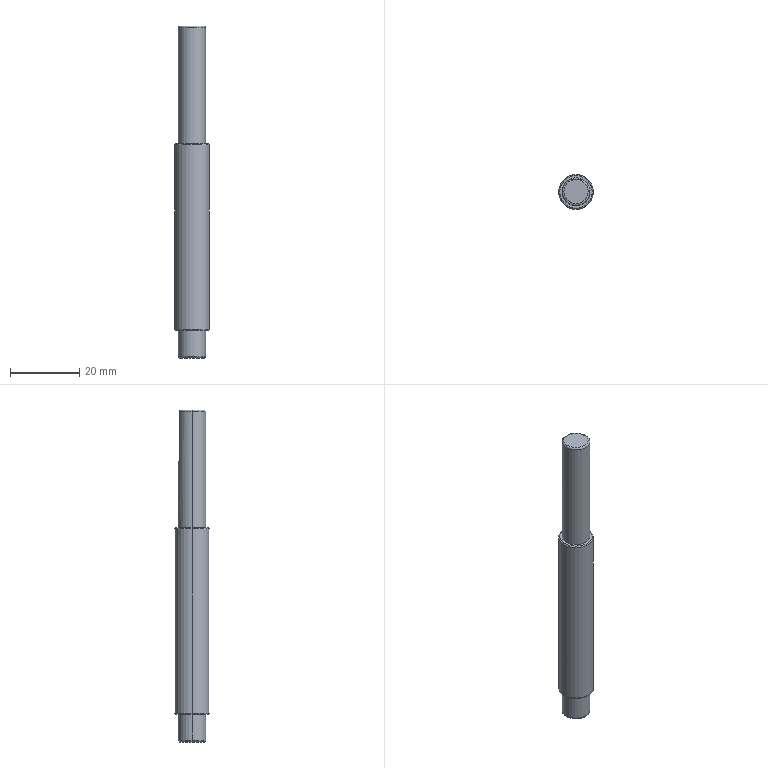Part | NX | features BREP 1 | 1 solid | 21 faces | box 10 x 10 x 95.8 mm | volume 6313 mm3 | torus 9 | cylinder 6 | plane 6 | commonest cylinder face diameters 8 x4 10 x2
STEP:
#1=CARTESIAN_POINT('',(-5.,0.,0.3));
#2=VERTEX_POINT('',#1);
#3=CARTESIAN_POINT('',(5.,0.,0.3));
#4=VERTEX_POINT('',#3);
#5=CARTESIAN_POINT('',(0.,0.,0.3));
#6=DIRECTION('',(0.,0.,1.));
#7=DIRECTION('',(-1.,0.,0.));
#8=AXIS2_PLACEMENT_3D('',#5,#6,#7);
#9=CIRCLE('',#8,5.);
#10=EDGE_CURVE('',#2,#4,#9,.T.);
#11=ORIENTED_EDGE('',*,*,#10,.F.);
#12=CARTESIAN_POINT('',(-4.7,0.,0.));
#13=VERTEX_POINT('',#12);
#14=CARTESIAN_POINT('',(-4.7,0.,0.3));
#15=DIRECTION('',(0.,-1.,0.));
#16=DIRECTION('',(-1.,0.,0.));
#17=AXIS2_PLACEMENT_3D('',#14,#15,#16);
#18=CIRCLE('',#17,0.3);
#19=EDGE_CURVE('',#2,#13,#18,.T.);
#20=ORIENTED_EDGE('',*,*,#19,.T.);
#21=CARTESIAN_POINT('',(4.7,0.,0.));
#22=VERTEX_POINT('',#21);
#23=CARTESIAN_POINT('',(0.,0.,0.));
#24=DIRECTION('',(0.,0.,1.));
#25=DIRECTION('',(-1.,0.,0.));
#26=AXIS2_PLACEMENT_3D('',#23,#24,#25);
#27=CIRCLE('',#26,4.7);
#28=EDGE_CURVE('',#13,#22,#27,.T.);
#29=ORIENTED_EDGE('',*,*,#28,.T.);
#30=CARTESIAN_POINT('',(4.7,0.,0.3));
#31=DIRECTION('',(0.,1.,0.));
#32=DIRECTION('',(1.,0.,0.));
#33=AXIS2_PLACEMENT_3D('',#30,#31,#32);
#34=CIRCLE('',#33,0.3);
#35=EDGE_CURVE('',#4,#22,#34,.T.);
#36=ORIENTED_EDGE('',*,*,#35,.F.);
#37=EDGE_LOOP('',(#11,#20,#29,#36));
#38=FACE_BOUND('',#37,.T.);
#39=CARTESIAN_POINT('',(0.,0.,0.3));
#40=DIRECTION('',(0.,0.,1.));
#41=DIRECTION('',(1.,0.,0.));
#42=AXIS2_PLACEMENT_3D('',#39,#40,#41);
#43=TOROIDAL_SURFACE('',#42,4.7,0.3);
#44=ADVANCED_FACE('',(#38),#43,.T.);
#45=CARTESIAN_POINT('',(4.7,0.,53.8));
#46=VERTEX_POINT('',#45);
#47=CARTESIAN_POINT('',(-4.7,0.,53.8));
#48=VERTEX_POINT('',#47);
#49=CARTESIAN_POINT('',(0.,0.,53.8));
#50=DIRECTION('',(0.,0.,-1.));
#51=DIRECTION('',(1.,0.,0.));
#52=AXIS2_PLACEMENT_3D('',#49,#50,#51);
#53=CIRCLE('',#52,4.7);
#54=EDGE_CURVE('',#46,#48,#53,.T.);
#55=ORIENTED_EDGE('',*,*,#54,.T.);
#56=CARTESIAN_POINT('',(-5.,0.,53.5));
#57=VERTEX_POINT('',#56);
#58=CARTESIAN_POINT('',(-4.7,0.,53.5));
#59=DIRECTION('',(0.,-1.,0.));
#60=DIRECTION('',(-1.,0.,0.));
#61=AXIS2_PLACEMENT_3D('',#58,#59,#60);
#62=CIRCLE('',#61,0.3);
#63=EDGE_CURVE('',#48,#57,#62,.T.);
#64=ORIENTED_EDGE('',*,*,#63,.T.);
#65=CARTESIAN_POINT('',(5.,0.,53.5));
#66=VERTEX_POINT('',#65);
#67=CARTESIAN_POINT('',(0.,0.,53.5));
#68=DIRECTION('',(0.,0.,-1.));
#69=DIRECTION('',(-1.,0.,0.));
#70=AXIS2_PLACEMENT_3D('',#67,#68,#69);
#71=CIRCLE('',#70,5.);
#72=EDGE_CURVE('',#66,#57,#71,.T.);
#73=ORIENTED_EDGE('',*,*,#72,.F.);
#74=CARTESIAN_POINT('',(4.7,0.,53.5));
#75=DIRECTION('',(0.,1.,0.));
#76=DIRECTION('',(1.,0.,0.));
#77=AXIS2_PLACEMENT_3D('',#74,#75,#76);
#78=CIRCLE('',#77,0.3);
#79=EDGE_CURVE('',#46,#66,#78,.T.);
#80=ORIENTED_EDGE('',*,*,#79,.F.);
#81=EDGE_LOOP('',(#55,#64,#73,#80));
#82=FACE_BOUND('',#81,.T.);
#83=CARTESIAN_POINT('',(0.,0.,53.5));
#84=DIRECTION('',(0.,0.,1.));
#85=DIRECTION('',(1.,0.,0.));
#86=AXIS2_PLACEMENT_3D('',#83,#84,#85);
#87=TOROIDAL_SURFACE('',#86,4.7,0.3);
#88=ADVANCED_FACE('',(#82),#87,.T.);
#89=CARTESIAN_POINT('',(-3.5,0.,-8.));
#90=VERTEX_POINT('',#89);
#91=CARTESIAN_POINT('',(3.5,0.,-8.));
#92=VERTEX_POINT('',#91);
#93=CARTESIAN_POINT('',(0.,0.,-8.));
#94=DIRECTION('',(0.,0.,1.));
#95=DIRECTION('',(-1.,0.,0.));
#96=AXIS2_PLACEMENT_3D('',#93,#94,#95);
#97=CIRCLE('',#96,3.5);
#98=EDGE_CURVE('',#90,#92,#97,.T.);
#99=ORIENTED_EDGE('',*,*,#98,.T.);
#100=CARTESIAN_POINT('',(4.,0.,-7.5));
#101=VERTEX_POINT('',#100);
#102=CARTESIAN_POINT('',(3.5,0.,-7.5));
#103=DIRECTION('',(0.,-1.,0.));
#104=DIRECTION('',(1.,0.,0.));
#105=AXIS2_PLACEMENT_3D('',#102,#103,#104);
#106=CIRCLE('',#105,0.5);
#107=EDGE_CURVE('',#101,#92,#106,.F.);
#108=ORIENTED_EDGE('',*,*,#107,.F.);
#109=CARTESIAN_POINT('',(-4.,0.,-7.5));
#110=VERTEX_POINT('',#109);
#111=CARTESIAN_POINT('',(0.,0.,-7.5));
#112=DIRECTION('',(0.,0.,1.));
#113=DIRECTION('',(1.,0.,0.));
#114=AXIS2_PLACEMENT_3D('',#111,#112,#113);
#115=CIRCLE('',#114,4.);
#116=EDGE_CURVE('',#110,#101,#115,.T.);
#117=ORIENTED_EDGE('',*,*,#116,.F.);
#118=CARTESIAN_POINT('',(-3.5,0.,-7.5));
#119=DIRECTION('',(0.,1.,0.));
#120=DIRECTION('',(-1.,0.,0.));
#121=AXIS2_PLACEMENT_3D('',#118,#119,#120);
#122=CIRCLE('',#121,0.5);
#123=EDGE_CURVE('',#110,#90,#122,.F.);
#124=ORIENTED_EDGE('',*,*,#123,.T.);
#125=EDGE_LOOP('',(#99,#108,#117,#124));
#126=FACE_BOUND('',#125,.T.);
#127=CARTESIAN_POINT('',(0.,0.,-7.5));
#128=DIRECTION('',(0.,0.,-1.));
#129=DIRECTION('',(-1.,0.,0.));
#130=AXIS2_PLACEMENT_3D('',#127,#128,#129);
#131=TOROIDAL_SURFACE('',#130,3.5,0.5);
#132=ADVANCED_FACE('',(#126),#131,.T.);
#133=CARTESIAN_POINT('',(3.5,0.,87.8));
#134=VERTEX_POINT('',#133);
#135=CARTESIAN_POINT('',(-3.5,0.,87.8));
#136=VERTEX_POINT('',#135);
#137=CARTESIAN_POINT('',(0.,0.,87.8));
#138=DIRECTION('',(0.,0.,-1.));
#139=DIRECTION('',(1.,0.,0.));
#140=AXIS2_PLACEMENT_3D('',#137,#138,#139);
#141=CIRCLE('',#140,3.5);
#142=EDGE_CURVE('',#134,#136,#141,.T.);
#143=ORIENTED_EDGE('',*,*,#142,.T.);
#144=CARTESIAN_POINT('',(-4.,0.,87.3));
#145=VERTEX_POINT('',#144);
#146=CARTESIAN_POINT('',(-3.5,0.,87.3));
#147=DIRECTION('',(0.,-1.,0.));
#148=DIRECTION('',(-1.,0.,0.));
#149=AXIS2_PLACEMENT_3D('',#146,#147,#148);
#150=CIRCLE('',#149,0.5);
#151=EDGE_CURVE('',#136,#145,#150,.T.);
#152=ORIENTED_EDGE('',*,*,#151,.T.);
#153=CARTESIAN_POINT('',(4.,0.,87.3));
#154=VERTEX_POINT('',#153);
#155=CARTESIAN_POINT('',(0.,0.,87.3));
#156=DIRECTION('',(0.,0.,-1.));
#157=DIRECTION('',(-1.,0.,0.));
#158=AXIS2_PLACEMENT_3D('',#155,#156,#157);
#159=CIRCLE('',#158,4.);
#160=EDGE_CURVE('',#154,#145,#159,.T.);
#161=ORIENTED_EDGE('',*,*,#160,.F.);
#162=CARTESIAN_POINT('',(3.5,0.,87.3));
#163=DIRECTION('',(0.,1.,0.));
#164=DIRECTION('',(1.,0.,0.));
#165=AXIS2_PLACEMENT_3D('',#162,#163,#164);
#166=CIRCLE('',#165,0.5);
#167=EDGE_CURVE('',#134,#154,#166,.T.);
#168=ORIENTED_EDGE('',*,*,#167,.F.);
#169=EDGE_LOOP('',(#143,#152,#161,#168));
#170=FACE_BOUND('',#169,.T.);
#171=CARTESIAN_POINT('',(0.,0.,87.3));
#172=DIRECTION('',(0.,0.,1.));
#173=DIRECTION('',(0.,-1.,0.));
#174=AXIS2_PLACEMENT_3D('',#171,#172,#173);
#175=TOROIDAL_SURFACE('',#174,3.5,0.5);
#176=ADVANCED_FACE('',(#170),#175,.T.);
#177=CARTESIAN_POINT('',(0.,3.5,87.8));
#178=VERTEX_POINT('',#177);
#179=CARTESIAN_POINT('',(0.,3.5,87.8));
#180=CARTESIAN_POINT('',(2.05,3.5,87.8));
#181=CARTESIAN_POINT('',(3.5,2.05,87.8));
#182=CARTESIAN_POINT('',(3.5,0.,87.8));
#183=(BOUNDED_CURVE()B_SPLINE_CURVE(3,(#179,#180,#181,#182),.UNSPECIFIED.,.F.,.F.)B_SPLINE_CURVE_WITH_KNOTS((4,4),(0.,1.),.PIECEWISE_BEZIER_KNOTS.)CURVE()GEOMETRIC_REPRESENTATION_ITEM()RATIONAL_B_SPLINE_CURVE((1.,0.8047,0.8047,1.))REPRESENTATION_ITEM(''));
#184=EDGE_CURVE('',#178,#134,#183,.T.);
#185=ORIENTED_EDGE('',*,*,#184,.T.);
#186=ORIENTED_EDGE('',*,*,#167,.T.);
#187=CARTESIAN_POINT('',(1.936,3.5,87.3));
#188=VERTEX_POINT('',#187);
#189=CARTESIAN_POINT('',(0.,0.,87.3));
#190=DIRECTION('',(0.,0.,-1.));
#191=DIRECTION('',(-1.,0.,0.));
#192=AXIS2_PLACEMENT_3D('',#189,#190,#191);
#193=CIRCLE('',#192,4.);
#194=EDGE_CURVE('',#188,#154,#193,.T.);
#195=ORIENTED_EDGE('',*,*,#194,.F.);
#196=CARTESIAN_POINT('',(1.936,3.5,87.3));
#197=CARTESIAN_POINT('',(1.936,3.5,87.482));
#198=CARTESIAN_POINT('',(1.58,3.5,87.71));
#199=CARTESIAN_POINT('',(0.8974,3.5,87.808));
#200=CARTESIAN_POINT('',(0.3553,3.5,87.8));
#201=CARTESIAN_POINT('',(0.,3.5,87.8));
#202=B_SPLINE_CURVE_WITH_KNOTS('',3,(#196,#197,#198,#199,#200,#201),.UNSPECIFIED.,.F.,.F.,(4,1,1,4),(0.,0.0005375,0.001075,0.00215),.UNSPECIFIED.);
#203=EDGE_CURVE('',#188,#178,#202,.T.);
#204=ORIENTED_EDGE('',*,*,#203,.T.);
#205=EDGE_LOOP('',(#185,#186,#195,#204));
#206=FACE_BOUND('',#205,.T.);
#207=CARTESIAN_POINT('',(0.,0.,87.3));
#208=DIRECTION('',(0.,0.,1.));
#209=DIRECTION('',(0.,-1.,0.));
#210=AXIS2_PLACEMENT_3D('',#207,#208,#209);
#211=TOROIDAL_SURFACE('',#210,3.5,0.5);
#212=ADVANCED_FACE('',(#206),#211,.T.);
#213=CARTESIAN_POINT('',(0.,0.,53.5));
#214=DIRECTION('',(0.,0.,-1.));
#215=DIRECTION('',(-1.,0.,0.));
#216=AXIS2_PLACEMENT_3D('',#213,#214,#215);
#217=CIRCLE('',#216,5.);
#218=EDGE_CURVE('',#57,#66,#217,.T.);
#219=ORIENTED_EDGE('',*,*,#218,.T.);
#220=CARTESIAN_POINT('',(5.,0.,53.8));
#221=DIRECTION('',(0.,0.,-1.));
#222=VECTOR('',#221,1000.);
#223=LINE('',#220,#222);
#224=EDGE_CURVE('',#4,#66,#223,.F.);
#225=ORIENTED_EDGE('',*,*,#224,.F.);
#226=CARTESIAN_POINT('',(0.,0.,0.3));
#227=DIRECTION('',(0.,0.,1.));
#228=DIRECTION('',(-1.,0.,0.));
#229=AXIS2_PLACEMENT_3D('',#226,#227,#228);
#230=CIRCLE('',#229,5.);
#231=EDGE_CURVE('',#4,#2,#230,.T.);
#232=ORIENTED_EDGE('',*,*,#231,.T.);
#233=CARTESIAN_POINT('',(-5.,0.,53.8));
#234=DIRECTION('',(0.,0.,-1.));
#235=VECTOR('',#234,1000.);
#236=LINE('',#233,#235);
#237=EDGE_CURVE('',#2,#57,#236,.F.);
#238=ORIENTED_EDGE('',*,*,#237,.T.);
#239=EDGE_LOOP('',(#219,#225,#232,#238));
#240=FACE_BOUND('',#239,.T.);
#241=CARTESIAN_POINT('',(0.,0.,53.8));
#242=DIRECTION('',(0.,0.,-1.));
#243=DIRECTION('',(1.,0.,0.));
#244=AXIS2_PLACEMENT_3D('',#241,#242,#243);
#245=CYLINDRICAL_SURFACE('',#244,5.);
#246=ADVANCED_FACE('',(#240),#245,.T.);
#247=CARTESIAN_POINT('',(0.,0.,-7.5));
#248=DIRECTION('',(0.,0.,1.));
#249=DIRECTION('',(1.,0.,0.));
#250=AXIS2_PLACEMENT_3D('',#247,#248,#249);
#251=CIRCLE('',#250,4.);
#252=EDGE_CURVE('',#101,#110,#251,.T.);
#253=ORIENTED_EDGE('',*,*,#252,.T.);
#254=CARTESIAN_POINT('',(-4.,0.,0.));
#255=VERTEX_POINT('',#254);
#256=CARTESIAN_POINT('',(-4.,0.,-8.));
#257=DIRECTION('',(0.,0.,1.));
#258=VECTOR('',#257,1000.);
#259=LINE('',#256,#258);
#260=EDGE_CURVE('',#110,#255,#259,.T.);
#261=ORIENTED_EDGE('',*,*,#260,.T.);
#262=CARTESIAN_POINT('',(4.,0.,0.));
#263=VERTEX_POINT('',#262);
#264=CARTESIAN_POINT('',(0.,0.,0.));
#265=DIRECTION('',(0.,0.,-1.));
#266=DIRECTION('',(1.,0.,0.));
#267=AXIS2_PLACEMENT_3D('',#264,#265,#266);
#268=CIRCLE('',#267,4.);
#269=EDGE_CURVE('',#255,#263,#268,.T.);
#270=ORIENTED_EDGE('',*,*,#269,.T.);
#271=CARTESIAN_POINT('',(4.,0.,-8.));
#272=DIRECTION('',(0.,0.,1.));
#273=VECTOR('',#272,1000.);
#274=LINE('',#271,#273);
#275=EDGE_CURVE('',#101,#263,#274,.T.);
#276=ORIENTED_EDGE('',*,*,#275,.F.);
#277=EDGE_LOOP('',(#253,#261,#270,#276));
#278=FACE_BOUND('',#277,.T.);
#279=CARTESIAN_POINT('',(0.,0.,-8.));
#280=DIRECTION('',(0.,0.,1.));
#281=DIRECTION('',(-1.,0.,0.));
#282=AXIS2_PLACEMENT_3D('',#279,#280,#281);
#283=CYLINDRICAL_SURFACE('',#282,4.);
#284=ADVANCED_FACE('',(#278),#283,.T.);
#285=ORIENTED_EDGE('',*,*,#194,.T.);
#286=CARTESIAN_POINT('',(4.,0.,53.8));
#287=VERTEX_POINT('',#286);
#288=CARTESIAN_POINT('',(4.,0.,87.8));
#289=DIRECTION('',(0.,0.,-1.));
#290=VECTOR('',#289,1000.);
#291=LINE('',#288,#290);
#292=EDGE_CURVE('',#287,#154,#291,.F.);
#293=ORIENTED_EDGE('',*,*,#292,.F.);
#294=CARTESIAN_POINT('',(-4.,0.,53.8));
#295=VERTEX_POINT('',#294);
#296=CARTESIAN_POINT('',(0.,0.,53.8));
#297=DIRECTION('',(0.,0.,-1.));
#298=DIRECTION('',(-1.,0.,0.));
#299=AXIS2_PLACEMENT_3D('',#296,#297,#298);
#300=CIRCLE('',#299,4.);
#301=EDGE_CURVE('',#295,#287,#300,.T.);
#302=ORIENTED_EDGE('',*,*,#301,.F.);
#303=CARTESIAN_POINT('',(-4.,0.,87.8));
#304=DIRECTION('',(0.,0.,-1.));
#305=VECTOR('',#304,1000.);
#306=LINE('',#303,#305);
#307=EDGE_CURVE('',#295,#145,#306,.F.);
#308=ORIENTED_EDGE('',*,*,#307,.T.);
#309=CARTESIAN_POINT('',(-1.936,3.5,87.3));
#310=VERTEX_POINT('',#309);
#311=CARTESIAN_POINT('',(0.,0.,87.3));
#312=DIRECTION('',(0.,0.,-1.));
#313=DIRECTION('',(-1.,0.,0.));
#314=AXIS2_PLACEMENT_3D('',#311,#312,#313);
#315=CIRCLE('',#314,4.);
#316=EDGE_CURVE('',#145,#310,#315,.T.);
#317=ORIENTED_EDGE('',*,*,#316,.T.);
#318=CARTESIAN_POINT('',(-1.936,3.5,72.8));
#319=VERTEX_POINT('',#318);
#320=CARTESIAN_POINT('',(-1.936,3.5,87.8));
#321=DIRECTION('',(0.,0.,-1.));
#322=VECTOR('',#321,1000.);
#323=LINE('',#320,#322);
#324=EDGE_CURVE('',#310,#319,#323,.T.);
#325=ORIENTED_EDGE('',*,*,#324,.T.);
#326=CARTESIAN_POINT('',(1.936,3.5,72.8));
#327=VERTEX_POINT('',#326);
#328=CARTESIAN_POINT('',(0.,0.,72.8));
#329=DIRECTION('',(0.,0.,-1.));
#330=DIRECTION('',(-1.,0.,0.));
#331=AXIS2_PLACEMENT_3D('',#328,#329,#330);
#332=CIRCLE('',#331,4.);
#333=EDGE_CURVE('',#319,#327,#332,.T.);
#334=ORIENTED_EDGE('',*,*,#333,.T.);
#335=CARTESIAN_POINT('',(1.936,3.5,87.8));
#336=DIRECTION('',(0.,0.,1.));
#337=VECTOR('',#336,1000.);
#338=LINE('',#335,#337);
#339=EDGE_CURVE('',#327,#188,#338,.T.);
#340=ORIENTED_EDGE('',*,*,#339,.T.);
#341=EDGE_LOOP('',(#285,#293,#302,#308,#317,#325,#334,#340));
#342=FACE_BOUND('',#341,.T.);
#343=CARTESIAN_POINT('',(0.,0.,87.8));
#344=DIRECTION('',(0.,0.,-1.));
#345=DIRECTION('',(1.,0.,0.));
#346=AXIS2_PLACEMENT_3D('',#343,#344,#345);
#347=CYLINDRICAL_SURFACE('',#346,4.);
#348=ADVANCED_FACE('',(#342),#347,.T.);
#349=ORIENTED_EDGE('',*,*,#224,.T.);
#350=ORIENTED_EDGE('',*,*,#72,.T.);
#351=ORIENTED_EDGE('',*,*,#237,.F.);
#352=ORIENTED_EDGE('',*,*,#10,.T.);
#353=EDGE_LOOP('',(#349,#350,#351,#352));
#354=FACE_BOUND('',#353,.T.);
#355=CARTESIAN_POINT('',(0.,0.,53.8));
#356=DIRECTION('',(0.,0.,-1.));
#357=DIRECTION('',(1.,0.,0.));
#358=AXIS2_PLACEMENT_3D('',#355,#356,#357);
#359=CYLINDRICAL_SURFACE('',#358,5.);
#360=ADVANCED_FACE('',(#354),#359,.T.);
#361=ORIENTED_EDGE('',*,*,#19,.F.);
#362=ORIENTED_EDGE('',*,*,#231,.F.);
#363=ORIENTED_EDGE('',*,*,#35,.T.);
#364=CARTESIAN_POINT('',(0.,0.,0.));
#365=DIRECTION('',(0.,0.,1.));
#366=DIRECTION('',(1.,0.,0.));
#367=AXIS2_PLACEMENT_3D('',#364,#365,#366);
#368=CIRCLE('',#367,4.7);
#369=EDGE_CURVE('',#22,#13,#368,.T.);
#370=ORIENTED_EDGE('',*,*,#369,.T.);
#371=EDGE_LOOP('',(#361,#362,#363,#370));
#372=FACE_BOUND('',#371,.T.);
#373=CARTESIAN_POINT('',(0.,0.,0.3));
#374=DIRECTION('',(0.,0.,1.));
#375=DIRECTION('',(1.,0.,0.));
#376=AXIS2_PLACEMENT_3D('',#373,#374,#375);
#377=TOROIDAL_SURFACE('',#376,4.7,0.3);
#378=ADVANCED_FACE('',(#372),#377,.T.);
#379=ORIENTED_EDGE('',*,*,#63,.F.);
#380=CARTESIAN_POINT('',(0.,0.,53.8));
#381=DIRECTION('',(0.,0.,-1.));
#382=DIRECTION('',(-1.,0.,0.));
#383=AXIS2_PLACEMENT_3D('',#380,#381,#382);
#384=CIRCLE('',#383,4.7);
#385=EDGE_CURVE('',#48,#46,#384,.T.);
#386=ORIENTED_EDGE('',*,*,#385,.T.);
#387=ORIENTED_EDGE('',*,*,#79,.T.);
#388=ORIENTED_EDGE('',*,*,#218,.F.);
#389=EDGE_LOOP('',(#379,#386,#387,#388));
#390=FACE_BOUND('',#389,.T.);
#391=CARTESIAN_POINT('',(0.,0.,53.5));
#392=DIRECTION('',(0.,0.,1.));
#393=DIRECTION('',(1.,0.,0.));
#394=AXIS2_PLACEMENT_3D('',#391,#392,#393);
#395=TOROIDAL_SURFACE('',#394,4.7,0.3);
#396=ADVANCED_FACE('',(#390),#395,.T.);
#397=CARTESIAN_POINT('',(0.,0.,0.));
#398=DIRECTION('',(0.,0.,-1.));
#399=DIRECTION('',(1.,0.,0.));
#400=AXIS2_PLACEMENT_3D('',#397,#398,#399);
#401=CIRCLE('',#400,4.);
#402=EDGE_CURVE('',#263,#255,#401,.T.);
#403=ORIENTED_EDGE('',*,*,#402,.F.);
#404=ORIENTED_EDGE('',*,*,#269,.F.);
#405=EDGE_LOOP('',(#403,#404));
#406=FACE_BOUND('',#405,.T.);
#407=ORIENTED_EDGE('',*,*,#369,.F.);
#408=ORIENTED_EDGE('',*,*,#28,.F.);
#409=EDGE_LOOP('',(#407,#408));
#410=FACE_BOUND('',#409,.T.);
#411=CARTESIAN_POINT('',(0.,0.,0.));
#412=DIRECTION('',(0.,0.,1.));
#413=DIRECTION('',(-1.,0.,0.));
#414=AXIS2_PLACEMENT_3D('',#411,#412,#413);
#415=PLANE('',#414);
#416=ADVANCED_FACE('',(#406,#410),#415,.F.);
#417=ORIENTED_EDGE('',*,*,#301,.T.);
#418=CARTESIAN_POINT('',(0.,0.,53.8));
#419=DIRECTION('',(0.,0.,-1.));
#420=DIRECTION('',(-1.,0.,0.));
#421=AXIS2_PLACEMENT_3D('',#418,#419,#420);
#422=CIRCLE('',#421,4.);
#423=EDGE_CURVE('',#287,#295,#422,.T.);
#424=ORIENTED_EDGE('',*,*,#423,.T.);
#425=EDGE_LOOP('',(#417,#424));
#426=FACE_BOUND('',#425,.T.);
#427=ORIENTED_EDGE('',*,*,#54,.F.);
#428=ORIENTED_EDGE('',*,*,#385,.F.);
#429=EDGE_LOOP('',(#427,#428));
#430=FACE_BOUND('',#429,.T.);
#431=CARTESIAN_POINT('',(0.,0.,53.8));
#432=DIRECTION('',(0.,0.,1.));
#433=DIRECTION('',(-1.,0.,0.));
#434=AXIS2_PLACEMENT_3D('',#431,#432,#433);
#435=PLANE('',#434);
#436=ADVANCED_FACE('',(#426,#430),#435,.T.);
#437=ORIENTED_EDGE('',*,*,#260,.F.);
#438=ORIENTED_EDGE('',*,*,#116,.T.);
#439=ORIENTED_EDGE('',*,*,#275,.T.);
#440=ORIENTED_EDGE('',*,*,#402,.T.);
#441=EDGE_LOOP('',(#437,#438,#439,#440));
#442=FACE_BOUND('',#441,.T.);
#443=CARTESIAN_POINT('',(0.,0.,-8.));
#444=DIRECTION('',(0.,0.,1.));
#445=DIRECTION('',(-1.,0.,0.));
#446=AXIS2_PLACEMENT_3D('',#443,#444,#445);
#447=CYLINDRICAL_SURFACE('',#446,4.);
#448=ADVANCED_FACE('',(#442),#447,.T.);
#449=ORIENTED_EDGE('',*,*,#292,.T.);
#450=ORIENTED_EDGE('',*,*,#160,.T.);
#451=ORIENTED_EDGE('',*,*,#307,.F.);
#452=ORIENTED_EDGE('',*,*,#423,.F.);
#453=EDGE_LOOP('',(#449,#450,#451,#452));
#454=FACE_BOUND('',#453,.T.);
#455=CARTESIAN_POINT('',(0.,0.,87.8));
#456=DIRECTION('',(0.,0.,-1.));
#457=DIRECTION('',(1.,0.,0.));
#458=AXIS2_PLACEMENT_3D('',#455,#456,#457);
#459=CYLINDRICAL_SURFACE('',#458,4.);
#460=ADVANCED_FACE('',(#454),#459,.T.);
#461=ORIENTED_EDGE('',*,*,#107,.T.);
#462=CARTESIAN_POINT('',(0.,0.,-8.));
#463=DIRECTION('',(0.,0.,1.));
#464=DIRECTION('',(1.,0.,0.));
#465=AXIS2_PLACEMENT_3D('',#462,#463,#464);
#466=CIRCLE('',#465,3.5);
#467=EDGE_CURVE('',#92,#90,#466,.T.);
#468=ORIENTED_EDGE('',*,*,#467,.T.);
#469=ORIENTED_EDGE('',*,*,#123,.F.);
#470=ORIENTED_EDGE('',*,*,#252,.F.);
#471=EDGE_LOOP('',(#461,#468,#469,#470));
#472=FACE_BOUND('',#471,.T.);
#473=CARTESIAN_POINT('',(0.,0.,-7.5));
#474=DIRECTION('',(0.,0.,-1.));
#475=DIRECTION('',(-1.,0.,0.));
#476=AXIS2_PLACEMENT_3D('',#473,#474,#475);
#477=TOROIDAL_SURFACE('',#476,3.5,0.5);
#478=ADVANCED_FACE('',(#472),#477,.T.);
#479=ORIENTED_EDGE('',*,*,#333,.F.);
#480=CARTESIAN_POINT('',(0.,3.5,72.8));
#481=DIRECTION('',(1.,0.,0.));
#482=VECTOR('',#481,1000.);
#483=LINE('',#480,#482);
#484=EDGE_CURVE('',#319,#327,#483,.T.);
#485=ORIENTED_EDGE('',*,*,#484,.T.);
#486=EDGE_LOOP('',(#479,#485));
#487=FACE_BOUND('',#486,.T.);
#488=CARTESIAN_POINT('',(0.,0.,72.8));
#489=DIRECTION('',(0.,0.,1.));
#490=DIRECTION('',(-1.,0.,0.));
#491=AXIS2_PLACEMENT_3D('',#488,#489,#490);
#492=PLANE('',#491);
#493=ADVANCED_FACE('',(#487),#492,.T.);
#494=ORIENTED_EDGE('',*,*,#203,.F.);
#495=ORIENTED_EDGE('',*,*,#339,.F.);
#496=ORIENTED_EDGE('',*,*,#484,.F.);
#497=ORIENTED_EDGE('',*,*,#324,.F.);
#498=CARTESIAN_POINT('',(0.,3.5,87.8));
#499=CARTESIAN_POINT('',(-0.3556,3.5,87.8));
#500=CARTESIAN_POINT('',(-0.8981,3.5,87.808));
#501=CARTESIAN_POINT('',(-1.583,3.5,87.709));
#502=CARTESIAN_POINT('',(-1.936,3.5,87.481));
#503=CARTESIAN_POINT('',(-1.936,3.5,87.3));
#504=B_SPLINE_CURVE_WITH_KNOTS('',3,(#498,#499,#500,#501,#502,#503),.UNSPECIFIED.,.F.,.F.,(4,1,1,4),(0.,0.001067,0.0016,0.002133),.UNSPECIFIED.);
#505=EDGE_CURVE('',#178,#310,#504,.T.);
#506=ORIENTED_EDGE('',*,*,#505,.F.);
#507=EDGE_LOOP('',(#494,#495,#496,#497,#506));
#508=FACE_BOUND('',#507,.T.);
#509=CARTESIAN_POINT('',(-1.936,3.5,72.8));
#510=DIRECTION('',(0.,-1.,0.));
#511=DIRECTION('',(0.,0.,1.));
#512=AXIS2_PLACEMENT_3D('',#509,#510,#511);
#513=PLANE('',#512);
#514=ADVANCED_FACE('',(#508),#513,.F.);
#515=ORIENTED_EDGE('',*,*,#151,.F.);
#516=CARTESIAN_POINT('',(-3.5,0.,87.8));
#517=CARTESIAN_POINT('',(-3.5,2.05,87.8));
#518=CARTESIAN_POINT('',(-2.05,3.5,87.8));
#519=CARTESIAN_POINT('',(0.,3.5,87.8));
#520=(BOUNDED_CURVE()B_SPLINE_CURVE(3,(#516,#517,#518,#519),.UNSPECIFIED.,.F.,.F.)B_SPLINE_CURVE_WITH_KNOTS((4,4),(0.,1.),.PIECEWISE_BEZIER_KNOTS.)CURVE()GEOMETRIC_REPRESENTATION_ITEM()RATIONAL_B_SPLINE_CURVE((1.,0.8047,0.8047,1.))REPRESENTATION_ITEM(''));
#521=EDGE_CURVE('',#136,#178,#520,.T.);
#522=ORIENTED_EDGE('',*,*,#521,.T.);
#523=ORIENTED_EDGE('',*,*,#505,.T.);
#524=ORIENTED_EDGE('',*,*,#316,.F.);
#525=EDGE_LOOP('',(#515,#522,#523,#524));
#526=FACE_BOUND('',#525,.T.);
#527=CARTESIAN_POINT('',(0.,0.,87.3));
#528=DIRECTION('',(0.,0.,1.));
#529=DIRECTION('',(0.,-1.,0.));
#530=AXIS2_PLACEMENT_3D('',#527,#528,#529);
#531=TOROIDAL_SURFACE('',#530,3.5,0.5);
#532=ADVANCED_FACE('',(#526),#531,.T.);
#533=ORIENTED_EDGE('',*,*,#98,.F.);
#534=ORIENTED_EDGE('',*,*,#467,.F.);
#535=EDGE_LOOP('',(#533,#534));
#536=FACE_BOUND('',#535,.T.);
#537=CARTESIAN_POINT('',(0.,0.,-8.));
#538=DIRECTION('',(0.,0.,-1.));
#539=DIRECTION('',(1.,0.,0.));
#540=AXIS2_PLACEMENT_3D('',#537,#538,#539);
#541=PLANE('',#540);
#542=ADVANCED_FACE('',(#536),#541,.T.);
#543=ORIENTED_EDGE('',*,*,#184,.F.);
#544=ORIENTED_EDGE('',*,*,#521,.F.);
#545=ORIENTED_EDGE('',*,*,#142,.F.);
#546=EDGE_LOOP('',(#543,#544,#545));
#547=FACE_BOUND('',#546,.T.);
#548=CARTESIAN_POINT('',(0.,0.,87.8));
#549=DIRECTION('',(0.,0.,1.));
#550=DIRECTION('',(-1.,0.,0.));
#551=AXIS2_PLACEMENT_3D('',#548,#549,#550);
#552=PLANE('',#551);
#553=ADVANCED_FACE('',(#547),#552,.T.);
#554=CLOSED_SHELL('',(#44,#88,#132,#176,#212,#246,#284,#348,#360,#378,#396,#416,#436,#448,#460,#478,#493,#514,#532,#542,#553));
#555=MANIFOLD_SOLID_BREP('',#554);
#556=(LENGTH_UNIT()NAMED_UNIT(*)SI_UNIT(.MILLI.,.METRE.));
#557=UNCERTAINTY_MEASURE_WITH_UNIT(LENGTH_MEASURE(0.0508),#556,'','');
#558=(NAMED_UNIT(*)PLANE_ANGLE_UNIT()SI_UNIT($,.RADIAN.));
#559=(NAMED_UNIT(*)SI_UNIT($,.STERADIAN.)SOLID_ANGLE_UNIT());
#560=(GEOMETRIC_REPRESENTATION_CONTEXT(3)GLOBAL_UNCERTAINTY_ASSIGNED_CONTEXT((#557))GLOBAL_UNIT_ASSIGNED_CONTEXT((#556,#558,#559))REPRESENTATION_CONTEXT('',''));
#561=ADVANCED_BREP_SHAPE_REPRESENTATION('',(#555),#560);